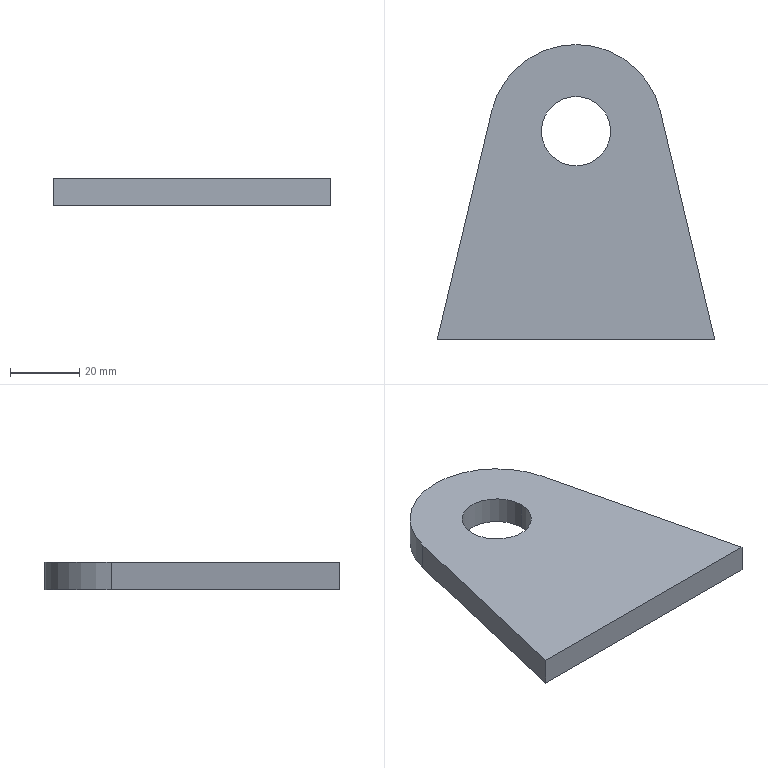Part | SolidWorks | features Extrusion 1 | 1 solid | 8 faces | box 80 x 85 x 8 mm | volume 36899 mm3 | plane 5 | cylinder 3 | commonest cylinder face diameters 20 x2 50 x1
STEP:
#1=CARTESIAN_POINT('',(30.,60.,8.));
#2=VERTEX_POINT('',#1);
#3=CARTESIAN_POINT('',(50.,60.,8.));
#4=VERTEX_POINT('',#3);
#5=CARTESIAN_POINT('',(40.,60.,8.));
#6=DIRECTION('',(0.,0.,1.));
#7=DIRECTION('',(1.,0.,0.));
#8=AXIS2_PLACEMENT_3D('',#5,#6,#7);
#9=CIRCLE('',#8,10.);
#10=EDGE_CURVE('',#2,#4,#9,.T.);
#11=ORIENTED_EDGE('',*,*,#10,.T.);
#12=CARTESIAN_POINT('',(50.,60.,0.));
#13=VERTEX_POINT('',#12);
#14=CARTESIAN_POINT('',(50.,60.,8.));
#15=DIRECTION('',(0.,0.,-1.));
#16=VECTOR('',#15,1000.);
#17=LINE('',#14,#16);
#18=EDGE_CURVE('',#4,#13,#17,.T.);
#19=ORIENTED_EDGE('',*,*,#18,.T.);
#20=CARTESIAN_POINT('',(30.,60.,0.));
#21=VERTEX_POINT('',#20);
#22=CARTESIAN_POINT('',(40.,60.,0.));
#23=DIRECTION('',(0.,0.,1.));
#24=DIRECTION('',(1.,0.,0.));
#25=AXIS2_PLACEMENT_3D('',#22,#23,#24);
#26=CIRCLE('',#25,10.);
#27=EDGE_CURVE('',#21,#13,#26,.T.);
#28=ORIENTED_EDGE('',*,*,#27,.F.);
#29=CARTESIAN_POINT('',(30.,60.,8.));
#30=DIRECTION('',(0.,0.,-1.));
#31=VECTOR('',#30,1000.);
#32=LINE('',#29,#31);
#33=EDGE_CURVE('',#2,#21,#32,.T.);
#34=ORIENTED_EDGE('',*,*,#33,.F.);
#35=EDGE_LOOP('',(#11,#19,#28,#34));
#36=FACE_OUTER_BOUND('',#35,.T.);
#37=CARTESIAN_POINT('',(40.,60.,8.));
#38=DIRECTION('',(0.,0.,-1.));
#39=DIRECTION('',(-1.,0.,0.));
#40=AXIS2_PLACEMENT_3D('',#37,#38,#39);
#41=CYLINDRICAL_SURFACE('',#40,10.);
#42=ADVANCED_FACE('',(#36),#41,.F.);
#43=CARTESIAN_POINT('',(15.681,65.796,8.));
#44=VERTEX_POINT('',#43);
#45=CARTESIAN_POINT('',(0.,0.,8.));
#46=VERTEX_POINT('',#45);
#47=CARTESIAN_POINT('',(0.,0.,8.));
#48=DIRECTION('',(-0.2318,-0.9728,0.));
#49=VECTOR('',#48,1000.);
#50=LINE('',#47,#49);
#51=EDGE_CURVE('',#44,#46,#50,.T.);
#52=ORIENTED_EDGE('',*,*,#51,.T.);
#53=CARTESIAN_POINT('',(80.,0.,8.));
#54=VERTEX_POINT('',#53);
#55=CARTESIAN_POINT('',(0.,0.,8.));
#56=DIRECTION('',(1.,0.,0.));
#57=VECTOR('',#56,1000.);
#58=LINE('',#55,#57);
#59=EDGE_CURVE('',#46,#54,#58,.T.);
#60=ORIENTED_EDGE('',*,*,#59,.T.);
#61=CARTESIAN_POINT('',(64.319,65.796,8.));
#62=VERTEX_POINT('',#61);
#63=CARTESIAN_POINT('',(80.,0.,8.));
#64=DIRECTION('',(-0.2318,0.9728,0.));
#65=VECTOR('',#64,1000.);
#66=LINE('',#63,#65);
#67=EDGE_CURVE('',#54,#62,#66,.T.);
#68=ORIENTED_EDGE('',*,*,#67,.T.);
#69=CARTESIAN_POINT('',(40.,60.,8.));
#70=DIRECTION('',(0.,0.,1.));
#71=DIRECTION('',(1.,0.,0.));
#72=AXIS2_PLACEMENT_3D('',#69,#70,#71);
#73=CIRCLE('',#72,25.);
#74=EDGE_CURVE('',#62,#44,#73,.T.);
#75=ORIENTED_EDGE('',*,*,#74,.T.);
#76=EDGE_LOOP('',(#52,#60,#68,#75));
#77=FACE_OUTER_BOUND('',#76,.T.);
#78=ORIENTED_EDGE('',*,*,#10,.F.);
#79=CARTESIAN_POINT('',(40.,60.,8.));
#80=DIRECTION('',(0.,0.,1.));
#81=DIRECTION('',(1.,0.,0.));
#82=AXIS2_PLACEMENT_3D('',#79,#80,#81);
#83=CIRCLE('',#82,10.);
#84=EDGE_CURVE('',#4,#2,#83,.T.);
#85=ORIENTED_EDGE('',*,*,#84,.F.);
#86=EDGE_LOOP('',(#78,#85));
#87=FACE_BOUND('',#86,.T.);
#88=CARTESIAN_POINT('',(40.,60.,8.));
#89=DIRECTION('',(0.,0.,1.));
#90=DIRECTION('',(1.,0.,0.));
#91=AXIS2_PLACEMENT_3D('',#88,#89,#90);
#92=PLANE('',#91);
#93=ADVANCED_FACE('',(#77,#87),#92,.T.);
#94=CARTESIAN_POINT('',(15.681,65.796,0.));
#95=VERTEX_POINT('',#94);
#96=CARTESIAN_POINT('',(0.,0.,0.));
#97=VERTEX_POINT('',#96);
#98=CARTESIAN_POINT('',(0.,0.,0.));
#99=DIRECTION('',(-0.2318,-0.9728,0.));
#100=VECTOR('',#99,1000.);
#101=LINE('',#98,#100);
#102=EDGE_CURVE('',#95,#97,#101,.T.);
#103=ORIENTED_EDGE('',*,*,#102,.F.);
#104=CARTESIAN_POINT('',(64.319,65.796,0.));
#105=VERTEX_POINT('',#104);
#106=CARTESIAN_POINT('',(40.,60.,0.));
#107=DIRECTION('',(0.,0.,1.));
#108=DIRECTION('',(1.,0.,0.));
#109=AXIS2_PLACEMENT_3D('',#106,#107,#108);
#110=CIRCLE('',#109,25.);
#111=EDGE_CURVE('',#105,#95,#110,.T.);
#112=ORIENTED_EDGE('',*,*,#111,.F.);
#113=CARTESIAN_POINT('',(80.,0.,0.));
#114=VERTEX_POINT('',#113);
#115=CARTESIAN_POINT('',(80.,0.,0.));
#116=DIRECTION('',(-0.2318,0.9728,0.));
#117=VECTOR('',#116,1000.);
#118=LINE('',#115,#117);
#119=EDGE_CURVE('',#114,#105,#118,.T.);
#120=ORIENTED_EDGE('',*,*,#119,.F.);
#121=CARTESIAN_POINT('',(0.,0.,0.));
#122=DIRECTION('',(1.,0.,0.));
#123=VECTOR('',#122,1000.);
#124=LINE('',#121,#123);
#125=EDGE_CURVE('',#97,#114,#124,.T.);
#126=ORIENTED_EDGE('',*,*,#125,.F.);
#127=EDGE_LOOP('',(#103,#112,#120,#126));
#128=FACE_OUTER_BOUND('',#127,.T.);
#129=ORIENTED_EDGE('',*,*,#27,.T.);
#130=CARTESIAN_POINT('',(40.,60.,0.));
#131=DIRECTION('',(0.,0.,1.));
#132=DIRECTION('',(1.,0.,0.));
#133=AXIS2_PLACEMENT_3D('',#130,#131,#132);
#134=CIRCLE('',#133,10.);
#135=EDGE_CURVE('',#13,#21,#134,.T.);
#136=ORIENTED_EDGE('',*,*,#135,.T.);
#137=EDGE_LOOP('',(#129,#136));
#138=FACE_BOUND('',#137,.T.);
#139=CARTESIAN_POINT('',(40.,60.,0.));
#140=DIRECTION('',(0.,0.,1.));
#141=DIRECTION('',(1.,0.,0.));
#142=AXIS2_PLACEMENT_3D('',#139,#140,#141);
#143=PLANE('',#142);
#144=ADVANCED_FACE('',(#128,#138),#143,.F.);
#145=ORIENTED_EDGE('',*,*,#102,.T.);
#146=CARTESIAN_POINT('',(0.,0.,8.));
#147=DIRECTION('',(0.,0.,-1.));
#148=VECTOR('',#147,1000.);
#149=LINE('',#146,#148);
#150=EDGE_CURVE('',#46,#97,#149,.T.);
#151=ORIENTED_EDGE('',*,*,#150,.F.);
#152=ORIENTED_EDGE('',*,*,#51,.F.);
#153=CARTESIAN_POINT('',(15.681,65.796,8.));
#154=DIRECTION('',(0.,0.,-1.));
#155=VECTOR('',#154,1000.);
#156=LINE('',#153,#155);
#157=EDGE_CURVE('',#44,#95,#156,.T.);
#158=ORIENTED_EDGE('',*,*,#157,.T.);
#159=EDGE_LOOP('',(#145,#151,#152,#158));
#160=FACE_OUTER_BOUND('',#159,.T.);
#161=CARTESIAN_POINT('',(0.,0.,8.));
#162=DIRECTION('',(0.9728,-0.2318,0.));
#163=DIRECTION('',(0.2318,0.9728,0.));
#164=AXIS2_PLACEMENT_3D('',#161,#162,#163);
#165=PLANE('',#164);
#166=ADVANCED_FACE('',(#160),#165,.F.);
#167=ORIENTED_EDGE('',*,*,#125,.T.);
#168=CARTESIAN_POINT('',(80.,0.,8.));
#169=DIRECTION('',(0.,0.,-1.));
#170=VECTOR('',#169,1000.);
#171=LINE('',#168,#170);
#172=EDGE_CURVE('',#54,#114,#171,.T.);
#173=ORIENTED_EDGE('',*,*,#172,.F.);
#174=ORIENTED_EDGE('',*,*,#59,.F.);
#175=ORIENTED_EDGE('',*,*,#150,.T.);
#176=EDGE_LOOP('',(#167,#173,#174,#175));
#177=FACE_OUTER_BOUND('',#176,.T.);
#178=CARTESIAN_POINT('',(0.,0.,8.));
#179=DIRECTION('',(0.,1.,0.));
#180=DIRECTION('',(0.,0.,1.));
#181=AXIS2_PLACEMENT_3D('',#178,#179,#180);
#182=PLANE('',#181);
#183=ADVANCED_FACE('',(#177),#182,.F.);
#184=ORIENTED_EDGE('',*,*,#119,.T.);
#185=CARTESIAN_POINT('',(64.319,65.796,8.));
#186=DIRECTION('',(0.,0.,-1.));
#187=VECTOR('',#186,1000.);
#188=LINE('',#185,#187);
#189=EDGE_CURVE('',#62,#105,#188,.T.);
#190=ORIENTED_EDGE('',*,*,#189,.F.);
#191=ORIENTED_EDGE('',*,*,#67,.F.);
#192=ORIENTED_EDGE('',*,*,#172,.T.);
#193=EDGE_LOOP('',(#184,#190,#191,#192));
#194=FACE_OUTER_BOUND('',#193,.T.);
#195=CARTESIAN_POINT('',(80.,0.,8.));
#196=DIRECTION('',(-0.9728,-0.2318,0.));
#197=DIRECTION('',(0.2318,-0.9728,0.));
#198=AXIS2_PLACEMENT_3D('',#195,#196,#197);
#199=PLANE('',#198);
#200=ADVANCED_FACE('',(#194),#199,.F.);
#201=ORIENTED_EDGE('',*,*,#111,.T.);
#202=ORIENTED_EDGE('',*,*,#157,.F.);
#203=ORIENTED_EDGE('',*,*,#74,.F.);
#204=ORIENTED_EDGE('',*,*,#189,.T.);
#205=EDGE_LOOP('',(#201,#202,#203,#204));
#206=FACE_OUTER_BOUND('',#205,.T.);
#207=CARTESIAN_POINT('',(40.,60.,8.));
#208=DIRECTION('',(0.,0.,-1.));
#209=DIRECTION('',(-1.,0.,0.));
#210=AXIS2_PLACEMENT_3D('',#207,#208,#209);
#211=CYLINDRICAL_SURFACE('',#210,25.);
#212=ADVANCED_FACE('',(#206),#211,.T.);
#213=ORIENTED_EDGE('',*,*,#18,.F.);
#214=ORIENTED_EDGE('',*,*,#84,.T.);
#215=ORIENTED_EDGE('',*,*,#33,.T.);
#216=ORIENTED_EDGE('',*,*,#135,.F.);
#217=EDGE_LOOP('',(#213,#214,#215,#216));
#218=FACE_OUTER_BOUND('',#217,.T.);
#219=CARTESIAN_POINT('',(40.,60.,8.));
#220=DIRECTION('',(0.,0.,-1.));
#221=DIRECTION('',(-1.,0.,0.));
#222=AXIS2_PLACEMENT_3D('',#219,#220,#221);
#223=CYLINDRICAL_SURFACE('',#222,10.);
#224=ADVANCED_FACE('',(#218),#223,.F.);
#225=CLOSED_SHELL('',(#42,#93,#144,#166,#183,#200,#212,#224));
#226=MANIFOLD_SOLID_BREP('',#225);
#227=CARTESIAN_POINT('',(0.,0.,0.));
#228=DIRECTION('',(0.,0.,1.));
#229=DIRECTION('',(1.,0.,0.));
#230=AXIS2_PLACEMENT_3D('',#227,#228,#229);
#231=(LENGTH_UNIT()NAMED_UNIT(*)SI_UNIT(.MILLI.,.METRE.));
#232=UNCERTAINTY_MEASURE_WITH_UNIT(LENGTH_MEASURE(0.00001),#231,'','');
#233=(NAMED_UNIT(*)PLANE_ANGLE_UNIT()SI_UNIT($,.RADIAN.));
#234=(NAMED_UNIT(*)SI_UNIT($,.STERADIAN.)SOLID_ANGLE_UNIT());
#235=(GEOMETRIC_REPRESENTATION_CONTEXT(3)GLOBAL_UNCERTAINTY_ASSIGNED_CONTEXT((#232))GLOBAL_UNIT_ASSIGNED_CONTEXT((#231,#233,#234))REPRESENTATION_CONTEXT('',''));
#236=ADVANCED_BREP_SHAPE_REPRESENTATION('',(#226,#230),#235);